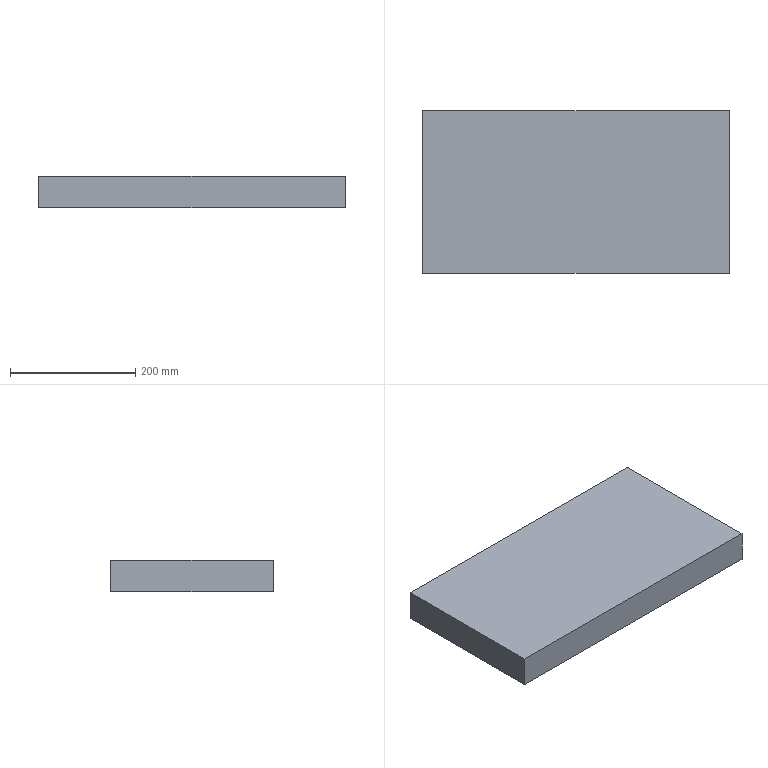Part | STEP file | 1 solid | 6 faces | box 489.379 x 259.164 x 50 mm | volume 6341468 mm3 | plane 6
STEP:
#1=CARTESIAN_POINT('',(0.,0.,0.));
#2=DIRECTION('',(0.,0.,1.));
#3=DIRECTION('',(1.,0.,0.));
#4=AXIS2_PLACEMENT_3D('',#1,#2,#3);
#5=CARTESIAN_POINT('',(-244.689,-240.836,393.641));
#6=VERTEX_POINT('',#5);
#7=CARTESIAN_POINT('',(-244.689,-500.,393.641));
#8=VERTEX_POINT('',#7);
#9=CARTESIAN_POINT('',(-244.689,-240.836,393.641));
#10=DIRECTION('',(0.,-1.,0.));
#11=VECTOR('',#10,1.);
#12=LINE('',#9,#11);
#13=CARTESIAN_POINT('',(-244.689,-240.836,343.641));
#14=DIRECTION('',(-1.,0.,0.));
#15=DIRECTION('',(0.,0.,1.));
#16=AXIS2_PLACEMENT_3D('',#13,#14,#15);
#17=PLANE('',#16);
#18=CARTESIAN_POINT('',(50.,0.));
#19=DIRECTION('',(0.,-1.));
#20=VECTOR('',#19,1.);
#21=LINE('',#18,#20);
#22=(GEOMETRIC_REPRESENTATION_CONTEXT(2)PARAMETRIC_REPRESENTATION_CONTEXT()REPRESENTATION_CONTEXT('',''));
#23=DEFINITIONAL_REPRESENTATION('',(#21),#22);
#24=PCURVE('',#17,#23);
#25=CARTESIAN_POINT('',(0.,0.,393.641));
#26=DIRECTION('',(0.,0.,1.));
#27=DIRECTION('',(1.,0.,0.));
#28=AXIS2_PLACEMENT_3D('',#25,#26,#27);
#29=PLANE('',#28);
#30=CARTESIAN_POINT('',(-244.689,-240.836));
#31=DIRECTION('',(0.,-1.));
#32=VECTOR('',#31,1.);
#33=LINE('',#30,#32);
#34=(GEOMETRIC_REPRESENTATION_CONTEXT(2)PARAMETRIC_REPRESENTATION_CONTEXT()REPRESENTATION_CONTEXT('',''));
#35=DEFINITIONAL_REPRESENTATION('',(#33),#34);
#36=PCURVE('',#29,#35);
#37=SURFACE_CURVE('',#12,(#24,#36),.PCURVE_S1.);
#38=EDGE_CURVE('',#6,#8,#37,.T.);
#39=ORIENTED_EDGE('',*,*,#38,.F.);
#40=CARTESIAN_POINT('',(-244.689,-240.836,343.641));
#41=VERTEX_POINT('',#40);
#42=CARTESIAN_POINT('',(-244.689,-240.836,343.641));
#43=DIRECTION('',(0.,0.,1.));
#44=VECTOR('',#43,1.);
#45=LINE('',#42,#44);
#46=CARTESIAN_POINT('',(0.,0.));
#47=DIRECTION('',(1.,0.));
#48=VECTOR('',#47,1.);
#49=LINE('',#46,#48);
#50=(GEOMETRIC_REPRESENTATION_CONTEXT(2)PARAMETRIC_REPRESENTATION_CONTEXT()REPRESENTATION_CONTEXT('',''));
#51=DEFINITIONAL_REPRESENTATION('',(#49),#50);
#52=PCURVE('',#17,#51);
#53=CARTESIAN_POINT('',(-244.689,-240.836,343.641));
#54=DIRECTION('',(0.,1.,0.));
#55=DIRECTION('',(0.,0.,1.));
#56=AXIS2_PLACEMENT_3D('',#53,#54,#55);
#57=PLANE('',#56);
#58=CARTESIAN_POINT('',(0.,0.));
#59=DIRECTION('',(1.,0.));
#60=VECTOR('',#59,1.);
#61=LINE('',#58,#60);
#62=(GEOMETRIC_REPRESENTATION_CONTEXT(2)PARAMETRIC_REPRESENTATION_CONTEXT()REPRESENTATION_CONTEXT('',''));
#63=DEFINITIONAL_REPRESENTATION('',(#61),#62);
#64=PCURVE('',#57,#63);
#65=SURFACE_CURVE('',#45,(#52,#64),.PCURVE_S1.);
#66=EDGE_CURVE('',#41,#6,#65,.T.);
#67=ORIENTED_EDGE('',*,*,#66,.F.);
#68=CARTESIAN_POINT('',(-244.689,-500.,343.641));
#69=VERTEX_POINT('',#68);
#70=CARTESIAN_POINT('',(-244.689,-240.836,343.641));
#71=DIRECTION('',(0.,-1.,0.));
#72=VECTOR('',#71,1.);
#73=LINE('',#70,#72);
#74=CARTESIAN_POINT('',(0.,0.));
#75=DIRECTION('',(0.,-1.));
#76=VECTOR('',#75,1.);
#77=LINE('',#74,#76);
#78=(GEOMETRIC_REPRESENTATION_CONTEXT(2)PARAMETRIC_REPRESENTATION_CONTEXT()REPRESENTATION_CONTEXT('',''));
#79=DEFINITIONAL_REPRESENTATION('',(#77),#78);
#80=PCURVE('',#17,#79);
#81=CARTESIAN_POINT('',(0.,0.,343.641));
#82=DIRECTION('',(0.,0.,1.));
#83=DIRECTION('',(1.,0.,0.));
#84=AXIS2_PLACEMENT_3D('',#81,#82,#83);
#85=PLANE('',#84);
#86=CARTESIAN_POINT('',(-244.689,-240.836));
#87=DIRECTION('',(0.,-1.));
#88=VECTOR('',#87,1.);
#89=LINE('',#86,#88);
#90=(GEOMETRIC_REPRESENTATION_CONTEXT(2)PARAMETRIC_REPRESENTATION_CONTEXT()REPRESENTATION_CONTEXT('',''));
#91=DEFINITIONAL_REPRESENTATION('',(#89),#90);
#92=PCURVE('',#85,#91);
#93=SURFACE_CURVE('',#73,(#80,#92),.PCURVE_S1.);
#94=EDGE_CURVE('',#41,#69,#93,.T.);
#95=ORIENTED_EDGE('',*,*,#94,.T.);
#96=CARTESIAN_POINT('',(-244.689,-500.,343.641));
#97=DIRECTION('',(0.,0.,1.));
#98=VECTOR('',#97,1.);
#99=LINE('',#96,#98);
#100=CARTESIAN_POINT('',(0.,-259.164));
#101=DIRECTION('',(1.,0.));
#102=VECTOR('',#101,1.);
#103=LINE('',#100,#102);
#104=(GEOMETRIC_REPRESENTATION_CONTEXT(2)PARAMETRIC_REPRESENTATION_CONTEXT()REPRESENTATION_CONTEXT('',''));
#105=DEFINITIONAL_REPRESENTATION('',(#103),#104);
#106=PCURVE('',#17,#105);
#107=CARTESIAN_POINT('',(-244.689,-500.,343.641));
#108=DIRECTION('',(0.,-1.,0.));
#109=DIRECTION('',(0.,0.,-1.));
#110=AXIS2_PLACEMENT_3D('',#107,#108,#109);
#111=PLANE('',#110);
#112=CARTESIAN_POINT('',(0.,0.));
#113=DIRECTION('',(-1.,0.));
#114=VECTOR('',#113,1.);
#115=LINE('',#112,#114);
#116=(GEOMETRIC_REPRESENTATION_CONTEXT(2)PARAMETRIC_REPRESENTATION_CONTEXT()REPRESENTATION_CONTEXT('',''));
#117=DEFINITIONAL_REPRESENTATION('',(#115),#116);
#118=PCURVE('',#111,#117);
#119=SURFACE_CURVE('',#99,(#106,#118),.PCURVE_S1.);
#120=EDGE_CURVE('',#69,#8,#119,.T.);
#121=ORIENTED_EDGE('',*,*,#120,.T.);
#122=EDGE_LOOP('',(#39,#67,#95,#121));
#123=FACE_BOUND('',#122,.T.);
#124=ADVANCED_FACE('',(#123),#17,.T.);
#125=CARTESIAN_POINT('',(244.689,-240.836,393.641));
#126=VERTEX_POINT('',#125);
#127=CARTESIAN_POINT('',(-244.689,-240.836,393.641));
#128=DIRECTION('',(-1.,0.,0.));
#129=VECTOR('',#128,1.);
#130=LINE('',#127,#129);
#131=CARTESIAN_POINT('',(50.,0.));
#132=DIRECTION('',(0.,-1.));
#133=VECTOR('',#132,1.);
#134=LINE('',#131,#133);
#135=(GEOMETRIC_REPRESENTATION_CONTEXT(2)PARAMETRIC_REPRESENTATION_CONTEXT()REPRESENTATION_CONTEXT('',''));
#136=DEFINITIONAL_REPRESENTATION('',(#134),#135);
#137=PCURVE('',#57,#136);
#138=CARTESIAN_POINT('',(-244.689,-240.836));
#139=DIRECTION('',(-1.,0.));
#140=VECTOR('',#139,1.);
#141=LINE('',#138,#140);
#142=(GEOMETRIC_REPRESENTATION_CONTEXT(2)PARAMETRIC_REPRESENTATION_CONTEXT()REPRESENTATION_CONTEXT('',''));
#143=DEFINITIONAL_REPRESENTATION('',(#141),#142);
#144=PCURVE('',#29,#143);
#145=SURFACE_CURVE('',#130,(#137,#144),.PCURVE_S1.);
#146=EDGE_CURVE('',#126,#6,#145,.T.);
#147=ORIENTED_EDGE('',*,*,#146,.F.);
#148=CARTESIAN_POINT('',(244.689,-240.836,343.641));
#149=VERTEX_POINT('',#148);
#150=CARTESIAN_POINT('',(244.689,-240.836,343.641));
#151=DIRECTION('',(0.,0.,1.));
#152=VECTOR('',#151,1.);
#153=LINE('',#150,#152);
#154=CARTESIAN_POINT('',(0.,489.379));
#155=DIRECTION('',(1.,0.));
#156=VECTOR('',#155,1.);
#157=LINE('',#154,#156);
#158=(GEOMETRIC_REPRESENTATION_CONTEXT(2)PARAMETRIC_REPRESENTATION_CONTEXT()REPRESENTATION_CONTEXT('',''));
#159=DEFINITIONAL_REPRESENTATION('',(#157),#158);
#160=PCURVE('',#57,#159);
#161=CARTESIAN_POINT('',(244.689,-240.836,343.641));
#162=DIRECTION('',(1.,0.,0.));
#163=DIRECTION('',(0.,0.,-1.));
#164=AXIS2_PLACEMENT_3D('',#161,#162,#163);
#165=PLANE('',#164);
#166=CARTESIAN_POINT('',(0.,0.));
#167=DIRECTION('',(-1.,0.));
#168=VECTOR('',#167,1.);
#169=LINE('',#166,#168);
#170=(GEOMETRIC_REPRESENTATION_CONTEXT(2)PARAMETRIC_REPRESENTATION_CONTEXT()REPRESENTATION_CONTEXT('',''));
#171=DEFINITIONAL_REPRESENTATION('',(#169),#170);
#172=PCURVE('',#165,#171);
#173=SURFACE_CURVE('',#153,(#160,#172),.PCURVE_S1.);
#174=EDGE_CURVE('',#149,#126,#173,.T.);
#175=ORIENTED_EDGE('',*,*,#174,.F.);
#176=CARTESIAN_POINT('',(-244.689,-240.836,343.641));
#177=DIRECTION('',(-1.,0.,0.));
#178=VECTOR('',#177,1.);
#179=LINE('',#176,#178);
#180=CARTESIAN_POINT('',(0.,0.));
#181=DIRECTION('',(0.,-1.));
#182=VECTOR('',#181,1.);
#183=LINE('',#180,#182);
#184=(GEOMETRIC_REPRESENTATION_CONTEXT(2)PARAMETRIC_REPRESENTATION_CONTEXT()REPRESENTATION_CONTEXT('',''));
#185=DEFINITIONAL_REPRESENTATION('',(#183),#184);
#186=PCURVE('',#57,#185);
#187=CARTESIAN_POINT('',(-244.689,-240.836));
#188=DIRECTION('',(-1.,0.));
#189=VECTOR('',#188,1.);
#190=LINE('',#187,#189);
#191=(GEOMETRIC_REPRESENTATION_CONTEXT(2)PARAMETRIC_REPRESENTATION_CONTEXT()REPRESENTATION_CONTEXT('',''));
#192=DEFINITIONAL_REPRESENTATION('',(#190),#191);
#193=PCURVE('',#85,#192);
#194=SURFACE_CURVE('',#179,(#186,#193),.PCURVE_S1.);
#195=EDGE_CURVE('',#149,#41,#194,.T.);
#196=ORIENTED_EDGE('',*,*,#195,.T.);
#197=ORIENTED_EDGE('',*,*,#66,.T.);
#198=EDGE_LOOP('',(#147,#175,#196,#197));
#199=FACE_BOUND('',#198,.T.);
#200=ADVANCED_FACE('',(#199),#57,.T.);
#201=CARTESIAN_POINT('',(244.689,-500.,393.641));
#202=VERTEX_POINT('',#201);
#203=CARTESIAN_POINT('',(244.689,-240.836,393.641));
#204=DIRECTION('',(0.,1.,0.));
#205=VECTOR('',#204,1.);
#206=LINE('',#203,#205);
#207=CARTESIAN_POINT('',(-50.,0.));
#208=DIRECTION('',(0.,1.));
#209=VECTOR('',#208,1.);
#210=LINE('',#207,#209);
#211=(GEOMETRIC_REPRESENTATION_CONTEXT(2)PARAMETRIC_REPRESENTATION_CONTEXT()REPRESENTATION_CONTEXT('',''));
#212=DEFINITIONAL_REPRESENTATION('',(#210),#211);
#213=PCURVE('',#165,#212);
#214=CARTESIAN_POINT('',(244.689,-240.836));
#215=DIRECTION('',(0.,1.));
#216=VECTOR('',#215,1.);
#217=LINE('',#214,#216);
#218=(GEOMETRIC_REPRESENTATION_CONTEXT(2)PARAMETRIC_REPRESENTATION_CONTEXT()REPRESENTATION_CONTEXT('',''));
#219=DEFINITIONAL_REPRESENTATION('',(#217),#218);
#220=PCURVE('',#29,#219);
#221=SURFACE_CURVE('',#206,(#213,#220),.PCURVE_S1.);
#222=EDGE_CURVE('',#202,#126,#221,.T.);
#223=ORIENTED_EDGE('',*,*,#222,.F.);
#224=CARTESIAN_POINT('',(244.689,-500.,343.641));
#225=VERTEX_POINT('',#224);
#226=CARTESIAN_POINT('',(244.689,-500.,343.641));
#227=DIRECTION('',(0.,0.,1.));
#228=VECTOR('',#227,1.);
#229=LINE('',#226,#228);
#230=CARTESIAN_POINT('',(0.,-259.164));
#231=DIRECTION('',(-1.,0.));
#232=VECTOR('',#231,1.);
#233=LINE('',#230,#232);
#234=(GEOMETRIC_REPRESENTATION_CONTEXT(2)PARAMETRIC_REPRESENTATION_CONTEXT()REPRESENTATION_CONTEXT('',''));
#235=DEFINITIONAL_REPRESENTATION('',(#233),#234);
#236=PCURVE('',#165,#235);
#237=CARTESIAN_POINT('',(0.,489.379));
#238=DIRECTION('',(-1.,0.));
#239=VECTOR('',#238,1.);
#240=LINE('',#237,#239);
#241=(GEOMETRIC_REPRESENTATION_CONTEXT(2)PARAMETRIC_REPRESENTATION_CONTEXT()REPRESENTATION_CONTEXT('',''));
#242=DEFINITIONAL_REPRESENTATION('',(#240),#241);
#243=PCURVE('',#111,#242);
#244=SURFACE_CURVE('',#229,(#236,#243),.PCURVE_S1.);
#245=EDGE_CURVE('',#225,#202,#244,.T.);
#246=ORIENTED_EDGE('',*,*,#245,.F.);
#247=CARTESIAN_POINT('',(244.689,-240.836,343.641));
#248=DIRECTION('',(0.,1.,0.));
#249=VECTOR('',#248,1.);
#250=LINE('',#247,#249);
#251=CARTESIAN_POINT('',(0.,0.));
#252=DIRECTION('',(0.,1.));
#253=VECTOR('',#252,1.);
#254=LINE('',#251,#253);
#255=(GEOMETRIC_REPRESENTATION_CONTEXT(2)PARAMETRIC_REPRESENTATION_CONTEXT()REPRESENTATION_CONTEXT('',''));
#256=DEFINITIONAL_REPRESENTATION('',(#254),#255);
#257=PCURVE('',#165,#256);
#258=CARTESIAN_POINT('',(244.689,-240.836));
#259=DIRECTION('',(0.,1.));
#260=VECTOR('',#259,1.);
#261=LINE('',#258,#260);
#262=(GEOMETRIC_REPRESENTATION_CONTEXT(2)PARAMETRIC_REPRESENTATION_CONTEXT()REPRESENTATION_CONTEXT('',''));
#263=DEFINITIONAL_REPRESENTATION('',(#261),#262);
#264=PCURVE('',#85,#263);
#265=SURFACE_CURVE('',#250,(#257,#264),.PCURVE_S1.);
#266=EDGE_CURVE('',#225,#149,#265,.T.);
#267=ORIENTED_EDGE('',*,*,#266,.T.);
#268=ORIENTED_EDGE('',*,*,#174,.T.);
#269=EDGE_LOOP('',(#223,#246,#267,#268));
#270=FACE_BOUND('',#269,.T.);
#271=ADVANCED_FACE('',(#270),#165,.T.);
#272=CARTESIAN_POINT('',(-244.689,-500.,393.641));
#273=DIRECTION('',(1.,0.,0.));
#274=VECTOR('',#273,1.);
#275=LINE('',#272,#274);
#276=CARTESIAN_POINT('',(-50.,0.));
#277=DIRECTION('',(0.,1.));
#278=VECTOR('',#277,1.);
#279=LINE('',#276,#278);
#280=(GEOMETRIC_REPRESENTATION_CONTEXT(2)PARAMETRIC_REPRESENTATION_CONTEXT()REPRESENTATION_CONTEXT('',''));
#281=DEFINITIONAL_REPRESENTATION('',(#279),#280);
#282=PCURVE('',#111,#281);
#283=CARTESIAN_POINT('',(-244.689,-500.));
#284=DIRECTION('',(1.,0.));
#285=VECTOR('',#284,1.);
#286=LINE('',#283,#285);
#287=(GEOMETRIC_REPRESENTATION_CONTEXT(2)PARAMETRIC_REPRESENTATION_CONTEXT()REPRESENTATION_CONTEXT('',''));
#288=DEFINITIONAL_REPRESENTATION('',(#286),#287);
#289=PCURVE('',#29,#288);
#290=SURFACE_CURVE('',#275,(#282,#289),.PCURVE_S1.);
#291=EDGE_CURVE('',#8,#202,#290,.T.);
#292=ORIENTED_EDGE('',*,*,#291,.F.);
#293=ORIENTED_EDGE('',*,*,#120,.F.);
#294=CARTESIAN_POINT('',(-244.689,-500.,343.641));
#295=DIRECTION('',(1.,0.,0.));
#296=VECTOR('',#295,1.);
#297=LINE('',#294,#296);
#298=CARTESIAN_POINT('',(0.,0.));
#299=DIRECTION('',(0.,1.));
#300=VECTOR('',#299,1.);
#301=LINE('',#298,#300);
#302=(GEOMETRIC_REPRESENTATION_CONTEXT(2)PARAMETRIC_REPRESENTATION_CONTEXT()REPRESENTATION_CONTEXT('',''));
#303=DEFINITIONAL_REPRESENTATION('',(#301),#302);
#304=PCURVE('',#111,#303);
#305=CARTESIAN_POINT('',(-244.689,-500.));
#306=DIRECTION('',(1.,0.));
#307=VECTOR('',#306,1.);
#308=LINE('',#305,#307);
#309=(GEOMETRIC_REPRESENTATION_CONTEXT(2)PARAMETRIC_REPRESENTATION_CONTEXT()REPRESENTATION_CONTEXT('',''));
#310=DEFINITIONAL_REPRESENTATION('',(#308),#309);
#311=PCURVE('',#85,#310);
#312=SURFACE_CURVE('',#297,(#304,#311),.PCURVE_S1.);
#313=EDGE_CURVE('',#69,#225,#312,.T.);
#314=ORIENTED_EDGE('',*,*,#313,.T.);
#315=ORIENTED_EDGE('',*,*,#245,.T.);
#316=EDGE_LOOP('',(#292,#293,#314,#315));
#317=FACE_BOUND('',#316,.T.);
#318=ADVANCED_FACE('',(#317),#111,.T.);
#319=ORIENTED_EDGE('',*,*,#94,.F.);
#320=ORIENTED_EDGE('',*,*,#195,.F.);
#321=ORIENTED_EDGE('',*,*,#266,.F.);
#322=ORIENTED_EDGE('',*,*,#313,.F.);
#323=EDGE_LOOP('',(#319,#320,#321,#322));
#324=FACE_BOUND('',#323,.T.);
#325=ADVANCED_FACE('',(#324),#85,.F.);
#326=ORIENTED_EDGE('',*,*,#38,.T.);
#327=ORIENTED_EDGE('',*,*,#291,.T.);
#328=ORIENTED_EDGE('',*,*,#222,.T.);
#329=ORIENTED_EDGE('',*,*,#146,.T.);
#330=EDGE_LOOP('',(#326,#327,#328,#329));
#331=FACE_BOUND('',#330,.T.);
#332=ADVANCED_FACE('',(#331),#29,.T.);
#333=CLOSED_SHELL('',(#124,#200,#271,#318,#325,#332));
#334=MANIFOLD_SOLID_BREP('',#333);
#335=(LENGTH_UNIT()NAMED_UNIT(*)SI_UNIT(.MILLI.,.METRE.));
#336=UNCERTAINTY_MEASURE_WITH_UNIT(LENGTH_MEASURE(0.0000001),#335,'','');
#337=(NAMED_UNIT(*)PLANE_ANGLE_UNIT()SI_UNIT($,.RADIAN.));
#338=(NAMED_UNIT(*)SI_UNIT($,.STERADIAN.)SOLID_ANGLE_UNIT());
#339=(GEOMETRIC_REPRESENTATION_CONTEXT(3)GLOBAL_UNCERTAINTY_ASSIGNED_CONTEXT((#336))GLOBAL_UNIT_ASSIGNED_CONTEXT((#335,#337,#338))REPRESENTATION_CONTEXT('',''));
#340=ADVANCED_BREP_SHAPE_REPRESENTATION('',(#4,#334),#339);